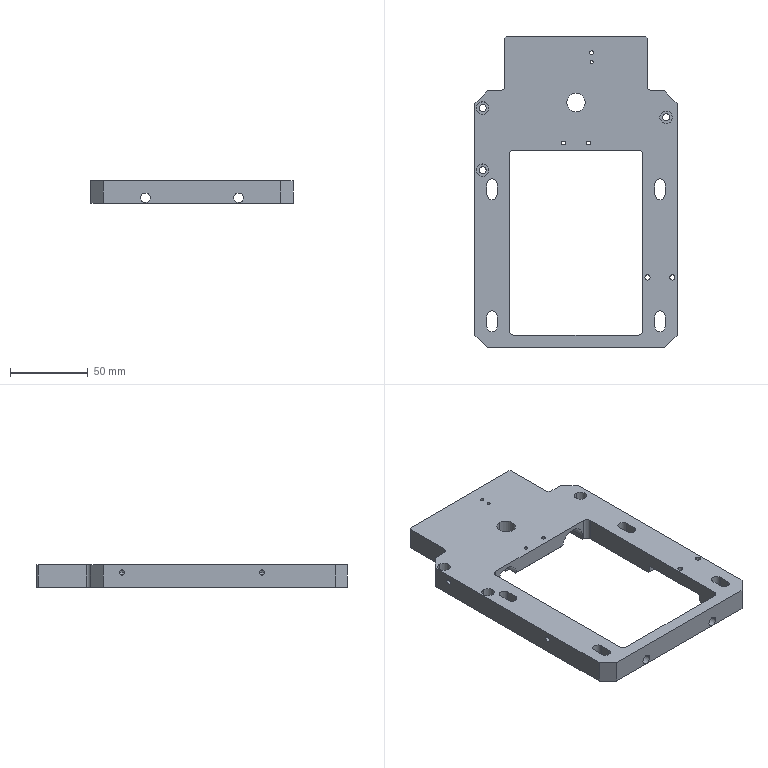NC program | NX | posted with a generic post | part box 130 x 200 x 14.5 mm
Lines 1 to 87 of 25347:
N10 G17 G21 G94 G90
(DRILLING , TOOL : ZXZ)
N12 T21 M6
N14 G54
N16 G17 G0 G90 X-55. Y46. B0. C0. S3500 M3
N18 G43 Z30. H21
N20 G94 G81 G98 Z-1. F250. R3.
N22 Y62.
N24 X48. Y58.
N26 X83.5 Y10.
N28 X89.5
N30 Y-6.5
N32 Y-14.5
N34 X57.5 Y0.
N36 X31.5 Y8.
N38 Y-8.
N40 X14. Y-60.
N42 X54.
N44 G80
N46 G0 X54. Y-60. Z30.
N48 M5
(DRILLING_COPY , TOOL : 4.5ZT)
N50 T12 M6
N52 G54
N54 G17 G0 G90 X14. Y-60. B0. C0. S2000 M3
N56 G43 Z30. H12
N58 G94 G83 G98 Z-15.852 F150. Q2. R3.
N60 X54.
N62 X57.5 Y0.
N64 X48. Y58.
N66 G80
N68 G0 X48. Y58. Z30.
N70 M5
(DRILLING_COPY_1 , TOOL : 3.3ZT)
N72 T13 M6
N74 G54
N76 G17 G0 G90 X-55. Y62. B0. C0. S2000 M3
N78 G43 Z30. H13
N80 G94 G83 G98 Z-16.991 F150. Q2. R3.
N82 Y46.
N84 G80
N86 G0 X-55. Y46. Z30.
N88 M5
(DRILLING_COPY_COPY , TOOL : 2.5ZT)
N90 T22 M6
N92 G54
N94 G17 G0 G90 X31.5 Y8. B0. C0. S2000 M3
N96 G43 Z30. H22
N98 G94 G83 G98 Z-16.751 F150. Q2. R3.
N100 Y-8.
N102 X89.5 Y10.
N104 G80
N106 G0 X89.5 Y10. Z30.
N108 M5
(DRILLING_COPY_1_COPY , TOOL : 1.6ZT)
N110 T24 M6
N112 G54
N114 G17 G0 G90 X83.5 Y10. B0. C0. S2000 M3
N116 G43 Z30. H24
N118 G94 G83 G98 Z-16.481 F100. Q2. R3.
N120 G80
N122 G0 X83.5 Y10. Z30.
N124 M5
(DRILLING_COPY_1_COPY_COPY , TOOL : 2.1ZT)
N126 T23 M6
N128 G54
N130 G17 G0 G90 X89.5 Y-6.5 B0. C0. S2000 M3
N132 G43 Z30. H23
N134 G94 G83 G98 Z-8.616 F100. Q2. R3.
N136 Y-14.5 Z-7.986
N138 G80
N140 G0 X89.5 Y-14.5 Z30.
N142 M5